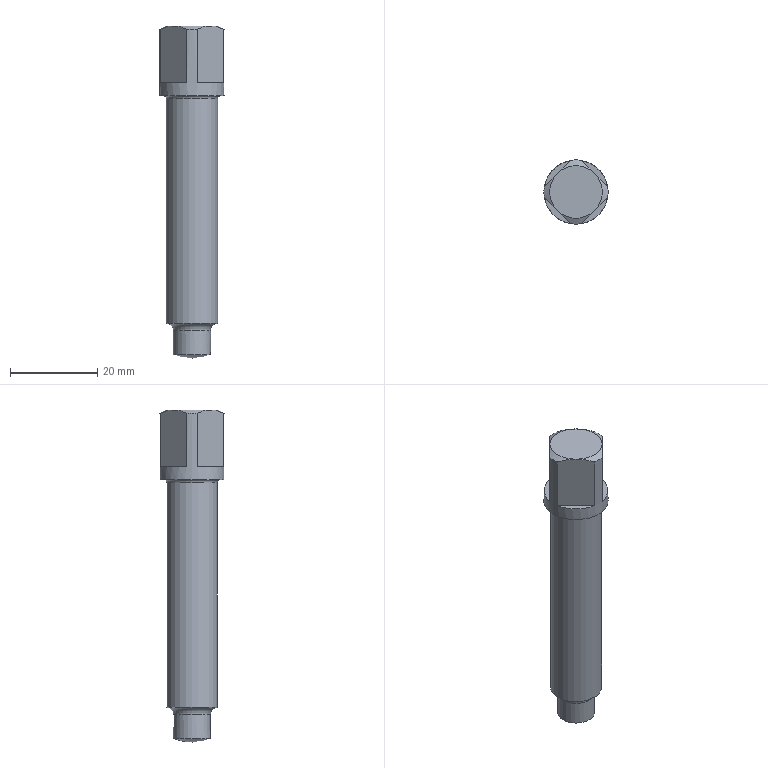Part | NX | features SKETCH 3, DATUM_CSYS 2, DATUM_PLANE 2, META 2, SWP104 2, EXTRUDE 1, LINE 1, SYMBOLIC_THREAD 1, THREADS 1 | 1 solid | 20 faces | box 14.7 x 14.7 x 76 mm | volume 8350 mm3 | plane 10 | cone 4 | cylinder 3 | torus 2 | sphere 1 | commonest cylinder face diameters 8.5 x1 11.701 x1 14.7 x1
STEP:
#1=CARTESIAN_POINT('',(-1.241,7.245,3.));
#2=VERTEX_POINT('',#1);
#3=CARTESIAN_POINT('',(-7.245,1.241,3.));
#4=VERTEX_POINT('',#3);
#5=CARTESIAN_POINT('',(-1.241,7.245,3.));
#6=DIRECTION('',(-0.7071,-0.7071,0.));
#7=VECTOR('',#6,1000.);
#8=LINE('',#5,#7);
#9=EDGE_CURVE('',#2,#4,#8,.T.);
#10=ORIENTED_EDGE('',*,*,#9,.F.);
#11=CARTESIAN_POINT('',(0.,0.,3.));
#12=DIRECTION('',(0.,0.,-1.));
#13=DIRECTION('',(-1.,0.,0.));
#14=AXIS2_PLACEMENT_3D('',#11,#12,#13);
#15=CIRCLE('',#14,7.35);
#16=EDGE_CURVE('',#4,#2,#15,.T.);
#17=ORIENTED_EDGE('',*,*,#16,.F.);
#18=EDGE_LOOP('',(#10,#17));
#19=FACE_BOUND('',#18,.T.);
#20=CARTESIAN_POINT('',(0.,0.,3.));
#21=DIRECTION('',(0.,0.,-1.));
#22=DIRECTION('',(-1.,0.,0.));
#23=AXIS2_PLACEMENT_3D('',#20,#21,#22);
#24=PLANE('',#23);
#25=ADVANCED_FACE('',(#19),#24,.F.);
#26=CARTESIAN_POINT('',(7.245,1.241,3.));
#27=VERTEX_POINT('',#26);
#28=CARTESIAN_POINT('',(1.241,7.245,3.));
#29=VERTEX_POINT('',#28);
#30=CARTESIAN_POINT('',(7.245,1.241,3.));
#31=DIRECTION('',(-0.7071,0.7071,0.));
#32=VECTOR('',#31,1000.);
#33=LINE('',#30,#32);
#34=EDGE_CURVE('',#27,#29,#33,.T.);
#35=ORIENTED_EDGE('',*,*,#34,.F.);
#36=CARTESIAN_POINT('',(0.,0.,3.));
#37=DIRECTION('',(0.,0.,-1.));
#38=DIRECTION('',(-1.,0.,0.));
#39=AXIS2_PLACEMENT_3D('',#36,#37,#38);
#40=CIRCLE('',#39,7.35);
#41=EDGE_CURVE('',#29,#27,#40,.T.);
#42=ORIENTED_EDGE('',*,*,#41,.F.);
#43=EDGE_LOOP('',(#35,#42));
#44=FACE_BOUND('',#43,.T.);
#45=CARTESIAN_POINT('',(0.,0.,3.));
#46=DIRECTION('',(0.,0.,-1.));
#47=DIRECTION('',(-1.,0.,0.));
#48=AXIS2_PLACEMENT_3D('',#45,#46,#47);
#49=PLANE('',#48);
#50=ADVANCED_FACE('',(#44),#49,.F.);
#51=CARTESIAN_POINT('',(1.241,-7.245,3.));
#52=VERTEX_POINT('',#51);
#53=CARTESIAN_POINT('',(7.245,-1.241,3.));
#54=VERTEX_POINT('',#53);
#55=CARTESIAN_POINT('',(1.241,-7.245,3.));
#56=DIRECTION('',(0.7071,0.7071,0.));
#57=VECTOR('',#56,1000.);
#58=LINE('',#55,#57);
#59=EDGE_CURVE('',#52,#54,#58,.T.);
#60=ORIENTED_EDGE('',*,*,#59,.F.);
#61=CARTESIAN_POINT('',(0.,0.,3.));
#62=DIRECTION('',(0.,0.,-1.));
#63=DIRECTION('',(-1.,0.,0.));
#64=AXIS2_PLACEMENT_3D('',#61,#62,#63);
#65=CIRCLE('',#64,7.35);
#66=EDGE_CURVE('',#54,#52,#65,.T.);
#67=ORIENTED_EDGE('',*,*,#66,.F.);
#68=EDGE_LOOP('',(#60,#67));
#69=FACE_BOUND('',#68,.T.);
#70=CARTESIAN_POINT('',(0.,0.,3.));
#71=DIRECTION('',(0.,0.,-1.));
#72=DIRECTION('',(-1.,0.,0.));
#73=AXIS2_PLACEMENT_3D('',#70,#71,#72);
#74=PLANE('',#73);
#75=ADVANCED_FACE('',(#69),#74,.F.);
#76=CARTESIAN_POINT('',(-7.245,-1.241,3.));
#77=VERTEX_POINT('',#76);
#78=CARTESIAN_POINT('',(-1.241,-7.245,3.));
#79=VERTEX_POINT('',#78);
#80=CARTESIAN_POINT('',(-7.245,-1.241,3.));
#81=DIRECTION('',(0.7071,-0.7071,0.));
#82=VECTOR('',#81,1000.);
#83=LINE('',#80,#82);
#84=EDGE_CURVE('',#77,#79,#83,.T.);
#85=ORIENTED_EDGE('',*,*,#84,.F.);
#86=CARTESIAN_POINT('',(0.,0.,3.));
#87=DIRECTION('',(0.,0.,-1.));
#88=DIRECTION('',(-1.,0.,0.));
#89=AXIS2_PLACEMENT_3D('',#86,#87,#88);
#90=CIRCLE('',#89,7.35);
#91=EDGE_CURVE('',#79,#77,#90,.T.);
#92=ORIENTED_EDGE('',*,*,#91,.F.);
#93=EDGE_LOOP('',(#85,#92));
#94=FACE_BOUND('',#93,.T.);
#95=CARTESIAN_POINT('',(0.,0.,3.));
#96=DIRECTION('',(0.,0.,-1.));
#97=DIRECTION('',(-1.,0.,0.));
#98=AXIS2_PLACEMENT_3D('',#95,#96,#97);
#99=PLANE('',#98);
#100=ADVANCED_FACE('',(#94),#99,.F.);
#101=CARTESIAN_POINT('',(-5.851,0.,-0.6));
#102=VERTEX_POINT('',#101);
#103=CARTESIAN_POINT('',(0.,0.,-0.6));
#104=DIRECTION('',(0.,0.,-1.));
#105=DIRECTION('',(-1.,0.,0.));
#106=AXIS2_PLACEMENT_3D('',#103,#104,#105);
#107=CIRCLE('',#106,5.851);
#108=EDGE_CURVE('',#102,#102,#107,.T.);
#109=ORIENTED_EDGE('',*,*,#108,.F.);
#110=EDGE_LOOP('',(#109));
#111=FACE_BOUND('',#110,.T.);
#112=CARTESIAN_POINT('',(-6.45,0.,0.));
#113=VERTEX_POINT('',#112);
#114=CARTESIAN_POINT('',(0.,0.,0.));
#115=DIRECTION('',(0.,0.,-1.));
#116=DIRECTION('',(-1.,0.,0.));
#117=AXIS2_PLACEMENT_3D('',#114,#115,#116);
#118=CIRCLE('',#117,6.45);
#119=EDGE_CURVE('',#113,#113,#118,.T.);
#120=ORIENTED_EDGE('',*,*,#119,.T.);
#121=EDGE_LOOP('',(#120));
#122=FACE_BOUND('',#121,.T.);
#123=CARTESIAN_POINT('',(0.,0.,-0.6));
#124=DIRECTION('',(0.,0.,-1.));
#125=DIRECTION('',(-1.,0.,0.));
#126=AXIS2_PLACEMENT_3D('',#123,#124,#125);
#127=TOROIDAL_SURFACE('',#126,6.45,0.6);
#128=ADVANCED_FACE('',(#111,#122),#127,.F.);
#129=CARTESIAN_POINT('',(-5.851,0.,-52.099));
#130=VERTEX_POINT('',#129);
#131=CARTESIAN_POINT('',(0.,0.,-52.099));
#132=DIRECTION('',(0.,0.,-1.));
#133=DIRECTION('',(-1.,0.,0.));
#134=AXIS2_PLACEMENT_3D('',#131,#132,#133);
#135=CIRCLE('',#134,5.851);
#136=EDGE_CURVE('',#130,#130,#135,.T.);
#137=ORIENTED_EDGE('',*,*,#136,.F.);
#138=EDGE_LOOP('',(#137));
#139=FACE_BOUND('',#138,.T.);
#140=ORIENTED_EDGE('',*,*,#108,.T.);
#141=EDGE_LOOP('',(#140));
#142=FACE_BOUND('',#141,.T.);
#143=CARTESIAN_POINT('',(0.,0.,0.));
#144=DIRECTION('',(0.,0.,-1.));
#145=DIRECTION('',(-1.,0.,0.));
#146=AXIS2_PLACEMENT_3D('',#143,#144,#145);
#147=CYLINDRICAL_SURFACE('',#146,5.851);
#148=ADVANCED_FACE('',(#139,#142),#147,.T.);
#149=CARTESIAN_POINT('',(-4.25,0.,-53.7));
#150=VERTEX_POINT('',#149);
#151=CARTESIAN_POINT('',(0.,0.,-53.7));
#152=DIRECTION('',(0.,0.,-1.));
#153=DIRECTION('',(-1.,0.,0.));
#154=AXIS2_PLACEMENT_3D('',#151,#152,#153);
#155=CIRCLE('',#154,4.25);
#156=EDGE_CURVE('',#150,#150,#155,.T.);
#157=ORIENTED_EDGE('',*,*,#156,.F.);
#158=EDGE_LOOP('',(#157));
#159=FACE_BOUND('',#158,.T.);
#160=ORIENTED_EDGE('',*,*,#136,.T.);
#161=EDGE_LOOP('',(#160));
#162=FACE_BOUND('',#161,.T.);
#163=CARTESIAN_POINT('',(0.,0.,-53.7));
#164=DIRECTION('',(0.,0.,-1.));
#165=DIRECTION('',(-1.,0.,0.));
#166=AXIS2_PLACEMENT_3D('',#163,#164,#165);
#167=TOROIDAL_SURFACE('',#166,5.851,1.601);
#168=ADVANCED_FACE('',(#159,#162),#167,.F.);
#169=CARTESIAN_POINT('',(-4.25,0.,-59.215));
#170=VERTEX_POINT('',#169);
#171=CARTESIAN_POINT('',(0.,0.,-59.215));
#172=DIRECTION('',(0.,0.,-1.));
#173=DIRECTION('',(-1.,0.,0.));
#174=AXIS2_PLACEMENT_3D('',#171,#172,#173);
#175=CIRCLE('',#174,4.25);
#176=EDGE_CURVE('',#170,#170,#175,.T.);
#177=ORIENTED_EDGE('',*,*,#176,.F.);
#178=EDGE_LOOP('',(#177));
#179=FACE_BOUND('',#178,.T.);
#180=ORIENTED_EDGE('',*,*,#156,.T.);
#181=EDGE_LOOP('',(#180));
#182=FACE_BOUND('',#181,.T.);
#183=CARTESIAN_POINT('',(0.,0.,0.));
#184=DIRECTION('',(0.,0.,-1.));
#185=DIRECTION('',(-1.,0.,0.));
#186=AXIS2_PLACEMENT_3D('',#183,#184,#185);
#187=CYLINDRICAL_SURFACE('',#186,4.25);
#188=ADVANCED_FACE('',(#179,#182),#187,.T.);
#189=ORIENTED_EDGE('',*,*,#176,.T.);
#190=EDGE_LOOP('',(#189));
#191=FACE_BOUND('',#190,.T.);
#192=CARTESIAN_POINT('',(0.,0.,-48.1));
#193=DIRECTION('',(0.,0.,-1.));
#194=DIRECTION('',(0.,1.,0.));
#195=AXIS2_PLACEMENT_3D('',#192,#193,#194);
#196=SPHERICAL_SURFACE('',#195,11.9);
#197=ADVANCED_FACE('',(#191),#196,.T.);
#198=CARTESIAN_POINT('',(-7.35,0.,0.));
#199=VERTEX_POINT('',#198);
#200=CARTESIAN_POINT('',(0.,0.,0.));
#201=DIRECTION('',(0.,0.,-1.));
#202=DIRECTION('',(-1.,0.,0.));
#203=AXIS2_PLACEMENT_3D('',#200,#201,#202);
#204=CIRCLE('',#203,7.35);
#205=EDGE_CURVE('',#199,#199,#204,.T.);
#206=ORIENTED_EDGE('',*,*,#205,.F.);
#207=EDGE_LOOP('',(#206));
#208=FACE_BOUND('',#207,.T.);
#209=CARTESIAN_POINT('',(-1.241,7.245,15.221));
#210=VERTEX_POINT('',#209);
#211=CARTESIAN_POINT('',(-1.241,7.245,16.));
#212=DIRECTION('',(0.,0.,-1.));
#213=VECTOR('',#212,1000.);
#214=LINE('',#211,#213);
#215=EDGE_CURVE('',#210,#2,#214,.T.);
#216=ORIENTED_EDGE('',*,*,#215,.F.);
#217=CARTESIAN_POINT('',(1.241,7.245,15.221));
#218=VERTEX_POINT('',#217);
#219=CARTESIAN_POINT('',(0.,0.,15.221));
#220=DIRECTION('',(0.,0.,-1.));
#221=DIRECTION('',(-1.,0.,0.));
#222=AXIS2_PLACEMENT_3D('',#219,#220,#221);
#223=CIRCLE('',#222,7.35);
#224=EDGE_CURVE('',#210,#218,#223,.T.);
#225=ORIENTED_EDGE('',*,*,#224,.T.);
#226=CARTESIAN_POINT('',(1.241,7.245,16.));
#227=DIRECTION('',(0.,0.,-1.));
#228=VECTOR('',#227,1000.);
#229=LINE('',#226,#228);
#230=EDGE_CURVE('',#218,#29,#229,.T.);
#231=ORIENTED_EDGE('',*,*,#230,.T.);
#232=ORIENTED_EDGE('',*,*,#41,.T.);
#233=CARTESIAN_POINT('',(7.245,1.241,15.221));
#234=VERTEX_POINT('',#233);
#235=CARTESIAN_POINT('',(7.245,1.241,16.));
#236=DIRECTION('',(0.,0.,-1.));
#237=VECTOR('',#236,1000.);
#238=LINE('',#235,#237);
#239=EDGE_CURVE('',#234,#27,#238,.T.);
#240=ORIENTED_EDGE('',*,*,#239,.F.);
#241=CARTESIAN_POINT('',(7.245,-1.241,15.221));
#242=VERTEX_POINT('',#241);
#243=CARTESIAN_POINT('',(0.,0.,15.221));
#244=DIRECTION('',(0.,0.,-1.));
#245=DIRECTION('',(-1.,0.,0.));
#246=AXIS2_PLACEMENT_3D('',#243,#244,#245);
#247=CIRCLE('',#246,7.35);
#248=EDGE_CURVE('',#234,#242,#247,.T.);
#249=ORIENTED_EDGE('',*,*,#248,.T.);
#250=CARTESIAN_POINT('',(7.245,-1.241,16.));
#251=DIRECTION('',(0.,0.,-1.));
#252=VECTOR('',#251,1000.);
#253=LINE('',#250,#252);
#254=EDGE_CURVE('',#242,#54,#253,.T.);
#255=ORIENTED_EDGE('',*,*,#254,.T.);
#256=ORIENTED_EDGE('',*,*,#66,.T.);
#257=CARTESIAN_POINT('',(1.241,-7.245,15.221));
#258=VERTEX_POINT('',#257);
#259=CARTESIAN_POINT('',(1.241,-7.245,16.));
#260=DIRECTION('',(0.,0.,-1.));
#261=VECTOR('',#260,1000.);
#262=LINE('',#259,#261);
#263=EDGE_CURVE('',#258,#52,#262,.T.);
#264=ORIENTED_EDGE('',*,*,#263,.F.);
#265=CARTESIAN_POINT('',(-1.241,-7.245,15.221));
#266=VERTEX_POINT('',#265);
#267=CARTESIAN_POINT('',(0.,0.,15.221));
#268=DIRECTION('',(0.,0.,-1.));
#269=DIRECTION('',(-1.,0.,0.));
#270=AXIS2_PLACEMENT_3D('',#267,#268,#269);
#271=CIRCLE('',#270,7.35);
#272=EDGE_CURVE('',#258,#266,#271,.T.);
#273=ORIENTED_EDGE('',*,*,#272,.T.);
#274=CARTESIAN_POINT('',(-1.241,-7.245,16.));
#275=DIRECTION('',(0.,0.,-1.));
#276=VECTOR('',#275,1000.);
#277=LINE('',#274,#276);
#278=EDGE_CURVE('',#266,#79,#277,.T.);
#279=ORIENTED_EDGE('',*,*,#278,.T.);
#280=ORIENTED_EDGE('',*,*,#91,.T.);
#281=CARTESIAN_POINT('',(-7.245,-1.241,15.221));
#282=VERTEX_POINT('',#281);
#283=CARTESIAN_POINT('',(-7.245,-1.241,16.));
#284=DIRECTION('',(0.,0.,-1.));
#285=VECTOR('',#284,1000.);
#286=LINE('',#283,#285);
#287=EDGE_CURVE('',#282,#77,#286,.T.);
#288=ORIENTED_EDGE('',*,*,#287,.F.);
#289=CARTESIAN_POINT('',(-7.245,1.241,15.221));
#290=VERTEX_POINT('',#289);
#291=CARTESIAN_POINT('',(0.,0.,15.221));
#292=DIRECTION('',(0.,0.,-1.));
#293=DIRECTION('',(-1.,0.,0.));
#294=AXIS2_PLACEMENT_3D('',#291,#292,#293);
#295=CIRCLE('',#294,7.35);
#296=EDGE_CURVE('',#282,#290,#295,.T.);
#297=ORIENTED_EDGE('',*,*,#296,.T.);
#298=CARTESIAN_POINT('',(-7.245,1.241,16.));
#299=DIRECTION('',(0.,0.,-1.));
#300=VECTOR('',#299,1000.);
#301=LINE('',#298,#300);
#302=EDGE_CURVE('',#290,#4,#301,.T.);
#303=ORIENTED_EDGE('',*,*,#302,.T.);
#304=ORIENTED_EDGE('',*,*,#16,.T.);
#305=EDGE_LOOP('',(#216,#225,#231,#232,#240,#249,#255,#256,#264,#273,#279,#280,#288,#297,#303,#304));
#306=FACE_BOUND('',#305,.T.);
#307=CARTESIAN_POINT('',(0.,0.,0.));
#308=DIRECTION('',(0.,0.,-1.));
#309=DIRECTION('',(-1.,0.,0.));
#310=AXIS2_PLACEMENT_3D('',#307,#308,#309);
#311=CYLINDRICAL_SURFACE('',#310,7.35);
#312=ADVANCED_FACE('',(#208,#306),#311,.T.);
#313=ORIENTED_EDGE('',*,*,#119,.F.);
#314=EDGE_LOOP('',(#313));
#315=FACE_BOUND('',#314,.T.);
#316=ORIENTED_EDGE('',*,*,#205,.T.);
#317=EDGE_LOOP('',(#316));
#318=FACE_BOUND('',#317,.T.);
#319=CARTESIAN_POINT('',(0.,7.35,0.));
#320=DIRECTION('',(0.,0.,1.));
#321=DIRECTION('',(1.,0.,0.));
#322=AXIS2_PLACEMENT_3D('',#319,#320,#321);
#323=PLANE('',#322);
#324=ADVANCED_FACE('',(#315,#318),#323,.F.);
#325=ORIENTED_EDGE('',*,*,#302,.F.);
#326=CARTESIAN_POINT('',(-4.243,4.243,16.));
#327=VERTEX_POINT('',#326);
#328=CARTESIAN_POINT('',(-7.245,1.241,15.221));
#329=CARTESIAN_POINT('',(-6.271,2.214,15.68));
#330=CARTESIAN_POINT('',(-5.268,3.218,16.));
#331=CARTESIAN_POINT('',(-4.243,4.243,16.));
#332=B_SPLINE_CURVE_WITH_KNOTS('',3,(#328,#329,#330,#331),.UNSPECIFIED.,.F.,.F.,(4,4),(0.000000627,0.004319),.UNSPECIFIED.);
#333=EDGE_CURVE('',#290,#327,#332,.T.);
#334=ORIENTED_EDGE('',*,*,#333,.T.);
#335=CARTESIAN_POINT('',(-4.243,4.243,16.));
#336=CARTESIAN_POINT('',(-3.211,5.274,16.));
#337=CARTESIAN_POINT('',(-2.217,6.268,15.681));
#338=CARTESIAN_POINT('',(-1.241,7.245,15.221));
#339=B_SPLINE_CURVE_WITH_KNOTS('',3,(#335,#336,#337,#338),.UNSPECIFIED.,.F.,.F.,(4,4),(0.004319,0.008665),.UNSPECIFIED.);
#340=EDGE_CURVE('',#327,#210,#339,.T.);
#341=ORIENTED_EDGE('',*,*,#340,.T.);
#342=ORIENTED_EDGE('',*,*,#215,.T.);
#343=ORIENTED_EDGE('',*,*,#9,.T.);
#344=EDGE_LOOP('',(#325,#334,#341,#342,#343));
#345=FACE_BOUND('',#344,.T.);
#346=CARTESIAN_POINT('',(-1.241,7.245,16.));
#347=DIRECTION('',(0.7071,-0.7071,0.));
#348=DIRECTION('',(0.7071,0.7071,0.));
#349=AXIS2_PLACEMENT_3D('',#346,#347,#348);
#350=PLANE('',#349);
#351=ADVANCED_FACE('',(#345),#350,.F.);
#352=ORIENTED_EDGE('',*,*,#278,.F.);
#353=CARTESIAN_POINT('',(-4.243,-4.243,16.));
#354=VERTEX_POINT('',#353);
#355=CARTESIAN_POINT('',(-1.241,-7.245,15.221));
#356=CARTESIAN_POINT('',(-2.214,-6.271,15.68));
#357=CARTESIAN_POINT('',(-3.218,-5.268,16.));
#358=CARTESIAN_POINT('',(-4.243,-4.243,16.));
#359=B_SPLINE_CURVE_WITH_KNOTS('',3,(#355,#356,#357,#358),.UNSPECIFIED.,.F.,.F.,(4,4),(0.000000627,0.004319),.UNSPECIFIED.);
#360=EDGE_CURVE('',#266,#354,#359,.T.);
#361=ORIENTED_EDGE('',*,*,#360,.T.);
#362=CARTESIAN_POINT('',(-4.243,-4.243,16.));
#363=CARTESIAN_POINT('',(-5.274,-3.211,16.));
#364=CARTESIAN_POINT('',(-6.268,-2.217,15.681));
#365=CARTESIAN_POINT('',(-7.245,-1.241,15.221));
#366=B_SPLINE_CURVE_WITH_KNOTS('',3,(#362,#363,#364,#365),.UNSPECIFIED.,.F.,.F.,(4,4),(0.004319,0.008665),.UNSPECIFIED.);
#367=EDGE_CURVE('',#354,#282,#366,.T.);
#368=ORIENTED_EDGE('',*,*,#367,.T.);
#369=ORIENTED_EDGE('',*,*,#287,.T.);
#370=ORIENTED_EDGE('',*,*,#84,.T.);
#371=EDGE_LOOP('',(#352,#361,#368,#369,#370));
#372=FACE_BOUND('',#371,.T.);
#373=CARTESIAN_POINT('',(-7.245,-1.241,16.));
#374=DIRECTION('',(0.7071,0.7071,0.));
#375=DIRECTION('',(-0.7071,0.7071,0.));
#376=AXIS2_PLACEMENT_3D('',#373,#374,#375);
#377=PLANE('',#376);
#378=ADVANCED_FACE('',(#372),#377,.F.);
#379=ORIENTED_EDGE('',*,*,#254,.F.);
#380=CARTESIAN_POINT('',(4.243,-4.243,16.));
#381=VERTEX_POINT('',#380);
#382=CARTESIAN_POINT('',(7.245,-1.241,15.221));
#383=CARTESIAN_POINT('',(6.271,-2.214,15.68));
#384=CARTESIAN_POINT('',(5.268,-3.218,16.));
#385=CARTESIAN_POINT('',(4.243,-4.243,16.));
#386=B_SPLINE_CURVE_WITH_KNOTS('',3,(#382,#383,#384,#385),.UNSPECIFIED.,.F.,.F.,(4,4),(0.000000627,0.004319),.UNSPECIFIED.);
#387=EDGE_CURVE('',#242,#381,#386,.T.);
#388=ORIENTED_EDGE('',*,*,#387,.T.);
#389=CARTESIAN_POINT('',(4.243,-4.243,16.));
#390=CARTESIAN_POINT('',(3.211,-5.274,16.));
#391=CARTESIAN_POINT('',(2.217,-6.268,15.681));
#392=CARTESIAN_POINT('',(1.241,-7.245,15.221));
#393=B_SPLINE_CURVE_WITH_KNOTS('',3,(#389,#390,#391,#392),.UNSPECIFIED.,.F.,.F.,(4,4),(0.004319,0.008665),.UNSPECIFIED.);
#394=EDGE_CURVE('',#381,#258,#393,.T.);
#395=ORIENTED_EDGE('',*,*,#394,.T.);
#396=ORIENTED_EDGE('',*,*,#263,.T.);
#397=ORIENTED_EDGE('',*,*,#59,.T.);
#398=EDGE_LOOP('',(#379,#388,#395,#396,#397));
#399=FACE_BOUND('',#398,.T.);
#400=CARTESIAN_POINT('',(1.241,-7.245,16.));
#401=DIRECTION('',(-0.7071,0.7071,0.));
#402=DIRECTION('',(-0.7071,-0.7071,0.));
#403=AXIS2_PLACEMENT_3D('',#400,#401,#402);
#404=PLANE('',#403);
#405=ADVANCED_FACE('',(#399),#404,.F.);
#406=ORIENTED_EDGE('',*,*,#230,.F.);
#407=CARTESIAN_POINT('',(4.243,4.243,16.));
#408=VERTEX_POINT('',#407);
#409=CARTESIAN_POINT('',(1.241,7.245,15.221));
#410=CARTESIAN_POINT('',(2.214,6.271,15.68));
#411=CARTESIAN_POINT('',(3.218,5.268,16.));
#412=CARTESIAN_POINT('',(4.243,4.243,16.));
#413=B_SPLINE_CURVE_WITH_KNOTS('',3,(#409,#410,#411,#412),.UNSPECIFIED.,.F.,.F.,(4,4),(0.000000627,0.004319),.UNSPECIFIED.);
#414=EDGE_CURVE('',#218,#408,#413,.T.);
#415=ORIENTED_EDGE('',*,*,#414,.T.);
#416=CARTESIAN_POINT('',(4.243,4.243,16.));
#417=CARTESIAN_POINT('',(5.274,3.211,16.));
#418=CARTESIAN_POINT('',(6.268,2.217,15.681));
#419=CARTESIAN_POINT('',(7.245,1.241,15.221));
#420=B_SPLINE_CURVE_WITH_KNOTS('',3,(#416,#417,#418,#419),.UNSPECIFIED.,.F.,.F.,(4,4),(0.004319,0.008665),.UNSPECIFIED.);
#421=EDGE_CURVE('',#408,#234,#420,.T.);
#422=ORIENTED_EDGE('',*,*,#421,.T.);
#423=ORIENTED_EDGE('',*,*,#239,.T.);
#424=ORIENTED_EDGE('',*,*,#34,.T.);
#425=EDGE_LOOP('',(#406,#415,#422,#423,#424));
#426=FACE_BOUND('',#425,.T.);
#427=CARTESIAN_POINT('',(7.245,1.241,16.));
#428=DIRECTION('',(-0.7071,-0.7071,0.));
#429=DIRECTION('',(0.7071,-0.7071,0.));
#430=AXIS2_PLACEMENT_3D('',#427,#428,#429);
#431=PLANE('',#430);
#432=ADVANCED_FACE('',(#426),#431,.F.);
#433=ORIENTED_EDGE('',*,*,#248,.F.);
#434=ORIENTED_EDGE('',*,*,#421,.F.);
#435=CARTESIAN_POINT('',(0.,0.,16.));
#436=DIRECTION('',(0.,0.,-1.));
#437=DIRECTION('',(-1.,0.,0.));
#438=AXIS2_PLACEMENT_3D('',#435,#436,#437);
#439=CIRCLE('',#438,6.);
#440=EDGE_CURVE('',#408,#381,#439,.T.);
#441=ORIENTED_EDGE('',*,*,#440,.T.);
#442=ORIENTED_EDGE('',*,*,#387,.F.);
#443=EDGE_LOOP('',(#433,#434,#441,#442));
#444=FACE_BOUND('',#443,.T.);
#445=CARTESIAN_POINT('',(0.,0.,16.));
#446=DIRECTION('',(0.,0.,-1.));
#447=DIRECTION('',(-1.,0.,0.));
#448=AXIS2_PLACEMENT_3D('',#445,#446,#447);
#449=CONICAL_SURFACE('',#448,6.,1.047);
#450=ADVANCED_FACE('',(#444),#449,.T.);
#451=CARTESIAN_POINT('',(0.,0.,16.));
#452=DIRECTION('',(0.,0.,-1.));
#453=DIRECTION('',(-1.,0.,0.));
#454=AXIS2_PLACEMENT_3D('',#451,#452,#453);
#455=CIRCLE('',#454,6.);
#456=EDGE_CURVE('',#327,#408,#455,.T.);
#457=ORIENTED_EDGE('',*,*,#456,.T.);
#458=ORIENTED_EDGE('',*,*,#414,.F.);
#459=ORIENTED_EDGE('',*,*,#224,.F.);
#460=ORIENTED_EDGE('',*,*,#340,.F.);
#461=EDGE_LOOP('',(#457,#458,#459,#460));
#462=FACE_BOUND('',#461,.T.);
#463=CARTESIAN_POINT('',(0.,0.,16.));
#464=DIRECTION('',(0.,0.,-1.));
#465=DIRECTION('',(-1.,0.,0.));
#466=AXIS2_PLACEMENT_3D('',#463,#464,#465);
#467=CONICAL_SURFACE('',#466,6.,1.047);
#468=ADVANCED_FACE('',(#462),#467,.T.);
#469=ORIENTED_EDGE('',*,*,#272,.F.);
#470=ORIENTED_EDGE('',*,*,#394,.F.);
#471=CARTESIAN_POINT('',(0.,0.,16.));
#472=DIRECTION('',(0.,0.,-1.));
#473=DIRECTION('',(-1.,0.,0.));
#474=AXIS2_PLACEMENT_3D('',#471,#472,#473);
#475=CIRCLE('',#474,6.);
#476=EDGE_CURVE('',#381,#354,#475,.T.);
#477=ORIENTED_EDGE('',*,*,#476,.T.);
#478=ORIENTED_EDGE('',*,*,#360,.F.);
#479=EDGE_LOOP('',(#469,#470,#477,#478));
#480=FACE_BOUND('',#479,.T.);
#481=CARTESIAN_POINT('',(0.,0.,16.));
#482=DIRECTION('',(0.,0.,-1.));
#483=DIRECTION('',(-1.,0.,0.));
#484=AXIS2_PLACEMENT_3D('',#481,#482,#483);
#485=CONICAL_SURFACE('',#484,6.,1.047);
#486=ADVANCED_FACE('',(#480),#485,.T.);
#487=ORIENTED_EDGE('',*,*,#296,.F.);
#488=ORIENTED_EDGE('',*,*,#367,.F.);
#489=CARTESIAN_POINT('',(0.,0.,16.));
#490=DIRECTION('',(0.,0.,-1.));
#491=DIRECTION('',(-1.,0.,0.));
#492=AXIS2_PLACEMENT_3D('',#489,#490,#491);
#493=CIRCLE('',#492,6.);
#494=EDGE_CURVE('',#354,#327,#493,.T.);
#495=ORIENTED_EDGE('',*,*,#494,.T.);
#496=ORIENTED_EDGE('',*,*,#333,.F.);
#497=EDGE_LOOP('',(#487,#488,#495,#496));
#498=FACE_BOUND('',#497,.T.);
#499=CARTESIAN_POINT('',(0.,0.,16.));
#500=DIRECTION('',(0.,0.,-1.));
#501=DIRECTION('',(-1.,0.,0.));
#502=AXIS2_PLACEMENT_3D('',#499,#500,#501);
#503=CONICAL_SURFACE('',#502,6.,1.047);
#504=ADVANCED_FACE('',(#498),#503,.T.);
#505=ORIENTED_EDGE('',*,*,#456,.F.);
#506=ORIENTED_EDGE('',*,*,#494,.F.);
#507=ORIENTED_EDGE('',*,*,#476,.F.);
#508=ORIENTED_EDGE('',*,*,#440,.F.);
#509=EDGE_LOOP('',(#505,#506,#507,#508));
#510=FACE_BOUND('',#509,.T.);
#511=CARTESIAN_POINT('',(0.,0.,16.));
#512=DIRECTION('',(0.,0.,1.));
#513=DIRECTION('',(1.,0.,0.));
#514=AXIS2_PLACEMENT_3D('',#511,#512,#513);
#515=PLANE('',#514);
#516=ADVANCED_FACE('',(#510),#515,.T.);
#517=CLOSED_SHELL('',(#25,#50,#75,#100,#128,#148,#168,#188,#197,#312,#324,#351,#378,#405,#432,#450,#468,#486,#504,#516));
#518=MANIFOLD_SOLID_BREP('',#517);
#519=(LENGTH_UNIT()NAMED_UNIT(*)SI_UNIT(.MILLI.,.METRE.));
#520=UNCERTAINTY_MEASURE_WITH_UNIT(LENGTH_MEASURE(0.0508),#519,'','');
#521=(NAMED_UNIT(*)PLANE_ANGLE_UNIT()SI_UNIT($,.RADIAN.));
#522=(NAMED_UNIT(*)SI_UNIT($,.STERADIAN.)SOLID_ANGLE_UNIT());
#523=(GEOMETRIC_REPRESENTATION_CONTEXT(3)GLOBAL_UNCERTAINTY_ASSIGNED_CONTEXT((#520))GLOBAL_UNIT_ASSIGNED_CONTEXT((#519,#521,#522))REPRESENTATION_CONTEXT('',''));
#524=ADVANCED_BREP_SHAPE_REPRESENTATION('',(#518),#523);